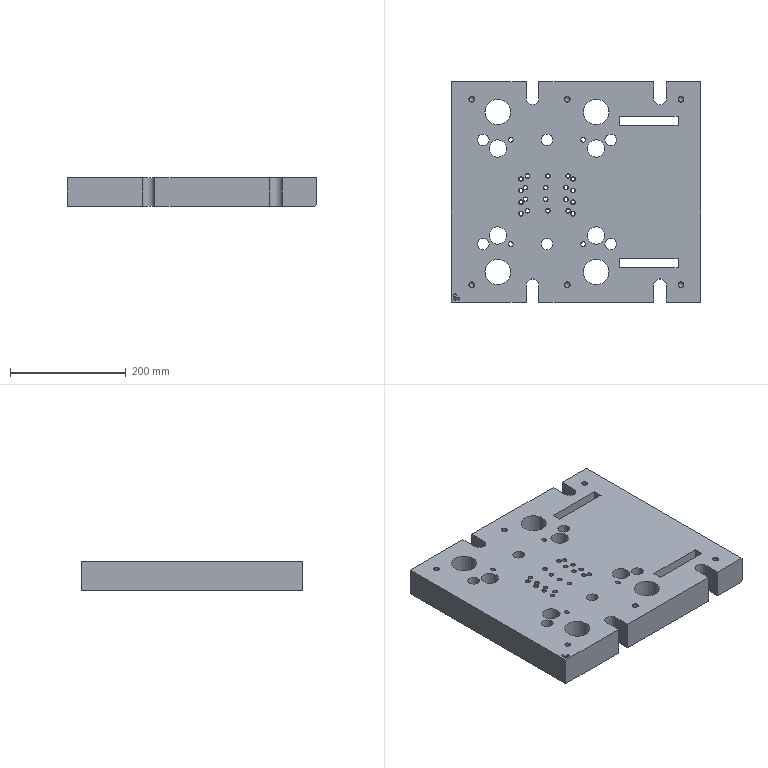Part | STEP file | 200 mesh_id2106 | 1 solid | 198 faces | box 430 x 380 x 50 mm | volume 6493004 mm3 | cone 79 | cylinder 77 | plane 38 | torus 4 | commonest cylinder face diameters 6.8 x28 26 x8 8.5 x6 20 x6 10 x5 5 x4